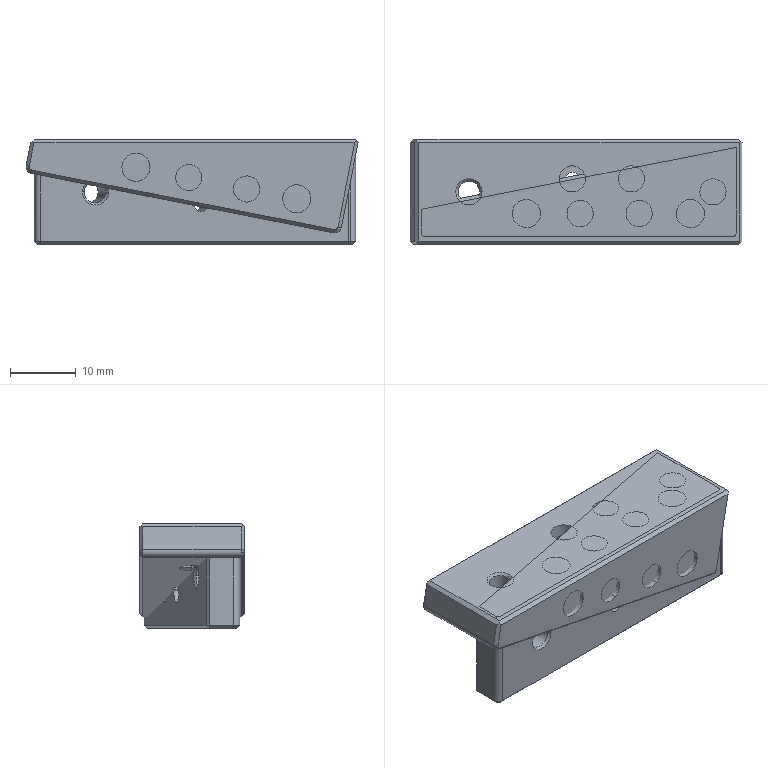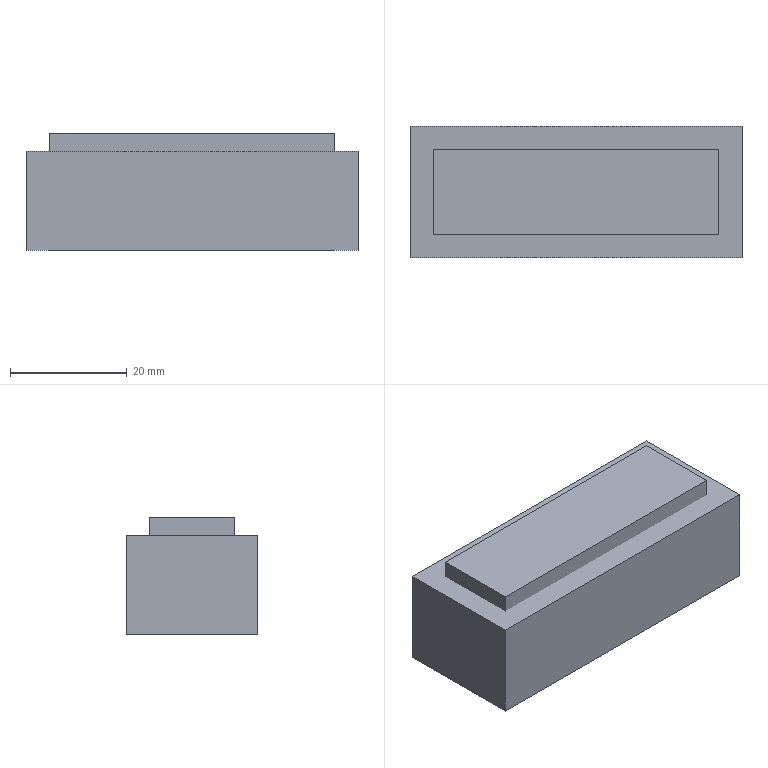CAM job | NX | 3-axis milling, drilling | part box 50.629 x 16.001 x 16.002 mm | stock box 56.985 x 22.6 x 20.002 mm
Tools:
number,name,description,diameter,corner_radius,flute_length,length,flutes
1,D63,Milling Tool-5 Parameters,63.0,0.0,50.0,75.0,2
2,D4A45,Milling Tool-5 Parameters,4.0,0.0,2.0,2.0,2
13,4.3ZT,Drilling Tool,3.3,0.0,35.0,50.0,2
10,D10,Milling Tool-5 Parameters,10.0,0.0,50.0,75.0,2
3,D3,Milling Tool-5 Parameters,3.0,0.0,50.0,75.0,2
16,3.3ZT,Drilling Tool,3.3,0.0,35.0,50.0,2
17,2.0ZT,Drilling Tool,2.0,0.0,35.0,50.0,2
Operations:
program,operation,operation_type,tool,method,geometry_group,spindle_rpm,surface_speed,feed_per_tooth,feed_cut,feed_plunge,cut_length_mm,path_length_mm,cut_time_min,machine_time_min
1虎钳,FLOOR_WALL,VolumeBased25DMillingOperation,D63,METHOD,A,6500.0,1286.0,0.0962,1250.0,100.0,131.985,185.985,0.1056,0.111
1虎钳,DRILLING_COPY,Operation,D4A45,METHOD,A,5000.0,62.0,0.025,250.0,0.0,16.0,144.028,0.064,0.0768
1虎钳,DRILLING_COPY_COPY_COPY_COPY_COPY_COPY,Operation,4.3ZT,METHOD,A,1910.0,21.0,0.0471,180.0,0.0,42.985,174.149,0.2388,0.2519
1虎钳,ADAPTIVE_MILLING,CavityMilling,D10,METHOD,A,9500.0,298.0,0.1579,3000.0,1000.0,1156.245,1242.246,0.3874,0.396
1虎钳,ZLEVEL_PROFILE_COPY_COPY_COPY_COPY,ZLevelMilling,D10,MILL_FINISH,A,9500.0,119.0,0.0632,1200.0,1000.0,154.772,243.773,0.1295,0.1384
1虎钳,HOLE_MILLING_1,CylinderMilling,D3,METHOD,A,9500.0,89.0,0.0632,1200.0,100.0,117.222,257.221,0.0977,0.1117
1虎钳,ZLEVEL_PROFILE_1_COPY_1_COPY_COPY,ZLevelMilling,D4A45,METHOD,A,9500.0,179.0,0.0526,1000.0,100.0,169.245,544.897,0.1692,0.2068
1虎钳,刀补6,CylinderMilling,D3,METHOD,A,9500.0,179.0,0.0632,1200.0,100.0,30.964,170.964,0.0258,0.0398
2,FLOOR_WALL_COPY,VolumeBased25DMillingOperation,D63,METHOD,B,6500.0,1286.0,0.0962,1250.0,100.0,619.926,1345.859,0.4959,0.5685
2,ZLEVEL_PROFILE_1_COPY_1_COPY_COPY_COPY,ZLevelMilling,D4A45,METHOD,B,9500.0,179.0,0.0526,1000.0,100.0,147.776,387.448,0.1478,0.1717
3-20层,DRILLING_COPY_COPY,Operation,D4A45,METHOD,C,5000.0,62.0,0.025,250.0,0.0,16.0,172.854,0.064,0.0797
3-20层,DRILLING_COPY_COPY_COPY_COPY_COPY_COPY_COPY,Operation,3.3ZT,METHOD,C,1910.0,21.0,0.0471,180.0,0.0,23.983,148.301,0.1332,0.1457
3-20层,DRILLING_COPY_COPY_COPY_COPY_COPY_COPY_COPY_COPY,Operation,2.0ZT,METHOD,C,1910.0,21.0,0.0471,180.0,0.0,35.108,142.703,0.195,0.2058
3-20层,HOLE_MILLING_1_COPY,CylinderMilling,D3,METHOD,C,9500.0,89.0,0.0632,1200.0,100.0,83.473,219.474,0.0696,0.0832
3-20层,ZLEVEL_PROFILE_1_COPY_1_COPY_COPY_COPY_1,ZLevelMilling,D4A45,METHOD,C,9500.0,179.0,0.0526,1000.0,100.0,42.873,367.136,0.0429,0.0753
3-20层,刀补6_COPY,CylinderMilling,D3,METHOD,C,9500.0,179.0,0.0632,1200.0,100.0,24.037,160.037,0.02,0.0336